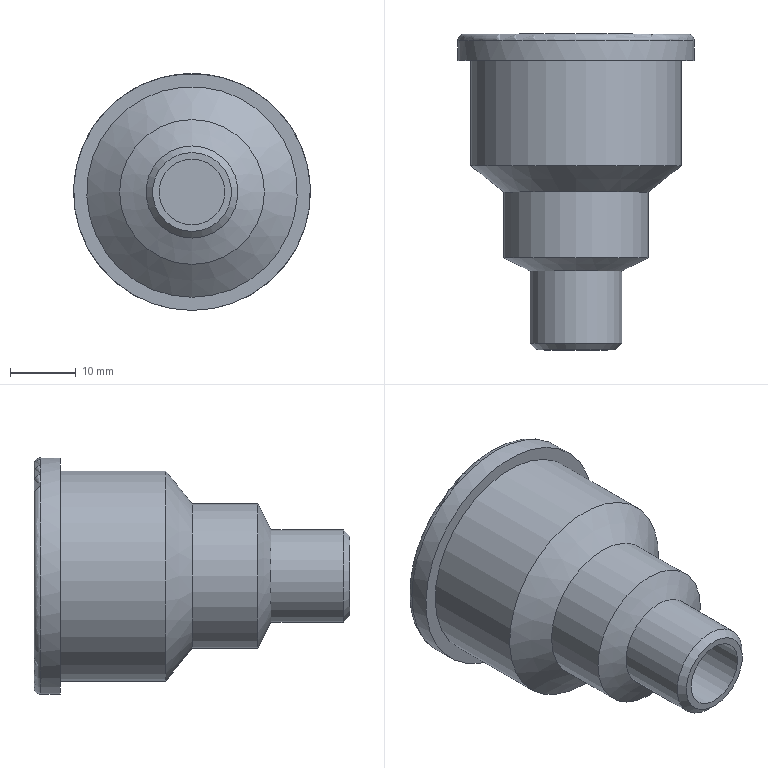Part | NX | features DATUM_CSYS 2, ABSOLUTE_DATUM_PLANE 1, BLEND 1, CHAMFER 1, SHELL 1, SKETCH 1, SWP104 1 | 1 solid | 17 faces | box 36 x 48 x 36 mm | volume 9367 mm3 | cylinder 7 | cone 5 | plane 4 | torus 1 | commonest cylinder face diameters 10 x1 14 x1 18 x1 22 x1 28 x1 32 x1
STEP:
#1=CARTESIAN_POINT('',(0.,-4.,-16.));
#2=VERTEX_POINT('',#1);
#3=CARTESIAN_POINT('',(0.,-4.,0.));
#4=DIRECTION('',(0.,-1.,0.));
#5=DIRECTION('',(0.,0.,-1.));
#6=AXIS2_PLACEMENT_3D('',#3,#4,#5);
#7=CIRCLE('',#6,16.);
#8=EDGE_CURVE('',#2,#2,#7,.T.);
#9=ORIENTED_EDGE('',*,*,#8,.T.);
#10=EDGE_LOOP('',(#9));
#11=FACE_BOUND('',#10,.T.);
#12=CARTESIAN_POINT('',(0.,-20.,-16.));
#13=VERTEX_POINT('',#12);
#14=CARTESIAN_POINT('',(0.,-20.,0.));
#15=DIRECTION('',(0.,-1.,0.));
#16=DIRECTION('',(0.,0.,-1.));
#17=AXIS2_PLACEMENT_3D('',#14,#15,#16);
#18=CIRCLE('',#17,16.);
#19=EDGE_CURVE('',#13,#13,#18,.T.);
#20=ORIENTED_EDGE('',*,*,#19,.F.);
#21=EDGE_LOOP('',(#20));
#22=FACE_BOUND('',#21,.T.);
#23=CARTESIAN_POINT('',(0.,0.,0.));
#24=DIRECTION('',(0.,-1.,0.));
#25=DIRECTION('',(0.,0.,-1.));
#26=AXIS2_PLACEMENT_3D('',#23,#24,#25);
#27=CYLINDRICAL_SURFACE('',#26,16.);
#28=ADVANCED_FACE('',(#11,#22),#27,.T.);
#29=CARTESIAN_POINT('',(0.,-4.,-18.));
#30=VERTEX_POINT('',#29);
#31=CARTESIAN_POINT('',(0.,-4.,0.));
#32=DIRECTION('',(0.,-1.,0.));
#33=DIRECTION('',(0.,0.,-1.));
#34=AXIS2_PLACEMENT_3D('',#31,#32,#33);
#35=CIRCLE('',#34,18.);
#36=EDGE_CURVE('',#30,#30,#35,.T.);
#37=ORIENTED_EDGE('',*,*,#36,.T.);
#38=EDGE_LOOP('',(#37));
#39=FACE_BOUND('',#38,.T.);
#40=ORIENTED_EDGE('',*,*,#8,.F.);
#41=EDGE_LOOP('',(#40));
#42=FACE_BOUND('',#41,.T.);
#43=CARTESIAN_POINT('',(16.,-4.,0.));
#44=DIRECTION('',(0.,-1.,0.));
#45=DIRECTION('',(0.,0.,-1.));
#46=AXIS2_PLACEMENT_3D('',#43,#44,#45);
#47=PLANE('',#46);
#48=ADVANCED_FACE('',(#39,#42),#47,.T.);
#49=CARTESIAN_POINT('',(0.,-1.,18.));
#50=VERTEX_POINT('',#49);
#51=CARTESIAN_POINT('',(0.,-1.,0.));
#52=DIRECTION('',(0.,1.,0.));
#53=DIRECTION('',(0.,0.,1.));
#54=AXIS2_PLACEMENT_3D('',#51,#52,#53);
#55=CIRCLE('',#54,18.);
#56=EDGE_CURVE('',#50,#50,#55,.F.);
#57=ORIENTED_EDGE('',*,*,#56,.T.);
#58=EDGE_LOOP('',(#57));
#59=FACE_BOUND('',#58,.T.);
#60=ORIENTED_EDGE('',*,*,#36,.F.);
#61=EDGE_LOOP('',(#60));
#62=FACE_BOUND('',#61,.T.);
#63=CARTESIAN_POINT('',(0.,0.,0.));
#64=DIRECTION('',(0.,-1.,0.));
#65=DIRECTION('',(0.,0.,-1.));
#66=AXIS2_PLACEMENT_3D('',#63,#64,#65);
#67=CYLINDRICAL_SURFACE('',#66,18.);
#68=ADVANCED_FACE('',(#59,#62),#67,.T.);
#69=CARTESIAN_POINT('',(0.,0.,17.));
#70=VERTEX_POINT('',#69);
#71=CARTESIAN_POINT('',(0.,0.,0.));
#72=DIRECTION('',(0.,1.,0.));
#73=DIRECTION('',(0.,0.,1.));
#74=AXIS2_PLACEMENT_3D('',#71,#72,#73);
#75=CIRCLE('',#74,17.);
#76=EDGE_CURVE('',#70,#70,#75,.T.);
#77=ORIENTED_EDGE('',*,*,#76,.T.);
#78=EDGE_LOOP('',(#77));
#79=FACE_BOUND('',#78,.T.);
#80=CARTESIAN_POINT('',(18.,0.,0.));
#81=DIRECTION('',(0.,1.,0.));
#82=DIRECTION('',(0.,0.,1.));
#83=AXIS2_PLACEMENT_3D('',#80,#81,#82);
#84=PLANE('',#83);
#85=ADVANCED_FACE('',(#79),#84,.T.);
#86=CARTESIAN_POINT('',(0.,-48.,-6.));
#87=VERTEX_POINT('',#86);
#88=CARTESIAN_POINT('',(0.,-48.,0.));
#89=DIRECTION('',(0.,-1.,0.));
#90=DIRECTION('',(0.,0.,-1.));
#91=AXIS2_PLACEMENT_3D('',#88,#89,#90);
#92=CIRCLE('',#91,6.);
#93=EDGE_CURVE('',#87,#87,#92,.T.);
#94=ORIENTED_EDGE('',*,*,#93,.T.);
#95=EDGE_LOOP('',(#94));
#96=FACE_BOUND('',#95,.T.);
#97=CARTESIAN_POINT('',(0.,-48.,-5.));
#98=VERTEX_POINT('',#97);
#99=CARTESIAN_POINT('',(0.,-48.,0.));
#100=DIRECTION('',(0.,-1.,0.));
#101=DIRECTION('',(0.,0.,-1.));
#102=AXIS2_PLACEMENT_3D('',#99,#100,#101);
#103=CIRCLE('',#102,5.);
#104=EDGE_CURVE('',#98,#98,#103,.T.);
#105=ORIENTED_EDGE('',*,*,#104,.F.);
#106=EDGE_LOOP('',(#105));
#107=FACE_BOUND('',#106,.T.);
#108=CARTESIAN_POINT('',(0.,-48.,0.));
#109=DIRECTION('',(0.,-1.,0.));
#110=DIRECTION('',(0.,0.,-1.));
#111=AXIS2_PLACEMENT_3D('',#108,#109,#110);
#112=PLANE('',#111);
#113=ADVANCED_FACE('',(#96,#107),#112,.T.);
#114=CARTESIAN_POINT('',(0.,-47.,-7.));
#115=VERTEX_POINT('',#114);
#116=CARTESIAN_POINT('',(0.,-47.,0.));
#117=DIRECTION('',(0.,-1.,0.));
#118=DIRECTION('',(0.,0.,-1.));
#119=AXIS2_PLACEMENT_3D('',#116,#117,#118);
#120=CIRCLE('',#119,7.);
#121=EDGE_CURVE('',#115,#115,#120,.F.);
#122=ORIENTED_EDGE('',*,*,#121,.T.);
#123=EDGE_LOOP('',(#122));
#124=FACE_BOUND('',#123,.T.);
#125=CARTESIAN_POINT('',(0.,-36.,-7.));
#126=VERTEX_POINT('',#125);
#127=CARTESIAN_POINT('',(0.,-36.,0.));
#128=DIRECTION('',(0.,-1.,0.));
#129=DIRECTION('',(0.,0.,-1.));
#130=AXIS2_PLACEMENT_3D('',#127,#128,#129);
#131=CIRCLE('',#130,7.);
#132=EDGE_CURVE('',#126,#126,#131,.T.);
#133=ORIENTED_EDGE('',*,*,#132,.T.);
#134=EDGE_LOOP('',(#133));
#135=FACE_BOUND('',#134,.T.);
#136=CARTESIAN_POINT('',(0.,0.,0.));
#137=DIRECTION('',(0.,-1.,0.));
#138=DIRECTION('',(0.,0.,-1.));
#139=AXIS2_PLACEMENT_3D('',#136,#137,#138);
#140=CYLINDRICAL_SURFACE('',#139,7.);
#141=ADVANCED_FACE('',(#124,#135),#140,.T.);
#142=CARTESIAN_POINT('',(0.,-34.,-11.));
#143=VERTEX_POINT('',#142);
#144=CARTESIAN_POINT('',(0.,-34.,0.));
#145=DIRECTION('',(0.,-1.,0.));
#146=DIRECTION('',(0.,0.,-1.));
#147=AXIS2_PLACEMENT_3D('',#144,#145,#146);
#148=CIRCLE('',#147,11.);
#149=EDGE_CURVE('',#143,#143,#148,.T.);
#150=ORIENTED_EDGE('',*,*,#149,.T.);
#151=EDGE_LOOP('',(#150));
#152=FACE_BOUND('',#151,.T.);
#153=ORIENTED_EDGE('',*,*,#132,.F.);
#154=EDGE_LOOP('',(#153));
#155=FACE_BOUND('',#154,.T.);
#156=CARTESIAN_POINT('',(0.,-36.,0.));
#157=DIRECTION('',(0.,1.,0.));
#158=DIRECTION('',(0.,0.,1.));
#159=AXIS2_PLACEMENT_3D('',#156,#157,#158);
#160=CONICAL_SURFACE('',#159,7.,1.107);
#161=ADVANCED_FACE('',(#152,#155),#160,.T.);
#162=CARTESIAN_POINT('',(0.,-24.,-11.));
#163=VERTEX_POINT('',#162);
#164=CARTESIAN_POINT('',(0.,-24.,0.));
#165=DIRECTION('',(0.,-1.,0.));
#166=DIRECTION('',(0.,0.,-1.));
#167=AXIS2_PLACEMENT_3D('',#164,#165,#166);
#168=CIRCLE('',#167,11.);
#169=EDGE_CURVE('',#163,#163,#168,.T.);
#170=ORIENTED_EDGE('',*,*,#169,.T.);
#171=EDGE_LOOP('',(#170));
#172=FACE_BOUND('',#171,.T.);
#173=ORIENTED_EDGE('',*,*,#149,.F.);
#174=EDGE_LOOP('',(#173));
#175=FACE_BOUND('',#174,.T.);
#176=CARTESIAN_POINT('',(0.,0.,0.));
#177=DIRECTION('',(0.,-1.,0.));
#178=DIRECTION('',(0.,0.,-1.));
#179=AXIS2_PLACEMENT_3D('',#176,#177,#178);
#180=CYLINDRICAL_SURFACE('',#179,11.);
#181=ADVANCED_FACE('',(#172,#175),#180,.T.);
#182=ORIENTED_EDGE('',*,*,#19,.T.);
#183=EDGE_LOOP('',(#182));
#184=FACE_BOUND('',#183,.T.);
#185=ORIENTED_EDGE('',*,*,#169,.F.);
#186=EDGE_LOOP('',(#185));
#187=FACE_BOUND('',#186,.T.);
#188=CARTESIAN_POINT('',(0.,-24.,0.));
#189=DIRECTION('',(0.,1.,0.));
#190=DIRECTION('',(0.,0.,1.));
#191=AXIS2_PLACEMENT_3D('',#188,#189,#190);
#192=CONICAL_SURFACE('',#191,11.,0.8961);
#193=ADVANCED_FACE('',(#184,#187),#192,.T.);
#194=CARTESIAN_POINT('',(0.,-2.,-14.));
#195=VERTEX_POINT('',#194);
#196=CARTESIAN_POINT('',(0.,-2.,0.));
#197=DIRECTION('',(0.,-1.,0.));
#198=DIRECTION('',(0.,0.,-1.));
#199=AXIS2_PLACEMENT_3D('',#196,#197,#198);
#200=CIRCLE('',#199,14.);
#201=EDGE_CURVE('',#195,#195,#200,.T.);
#202=ORIENTED_EDGE('',*,*,#201,.F.);
#203=EDGE_LOOP('',(#202));
#204=FACE_BOUND('',#203,.T.);
#205=CARTESIAN_POINT('',(0.,-19.039,14.));
#206=VERTEX_POINT('',#205);
#207=CARTESIAN_POINT('',(0.,-19.039,0.));
#208=DIRECTION('',(0.,1.,0.));
#209=DIRECTION('',(0.,0.,1.));
#210=AXIS2_PLACEMENT_3D('',#207,#208,#209);
#211=CIRCLE('',#210,14.);
#212=EDGE_CURVE('',#206,#206,#211,.F.);
#213=ORIENTED_EDGE('',*,*,#212,.T.);
#214=EDGE_LOOP('',(#213));
#215=FACE_BOUND('',#214,.T.);
#216=CARTESIAN_POINT('',(0.,0.,0.));
#217=DIRECTION('',(0.,-1.,0.));
#218=DIRECTION('',(0.,0.,-1.));
#219=AXIS2_PLACEMENT_3D('',#216,#217,#218);
#220=CYLINDRICAL_SURFACE('',#219,14.);
#221=ADVANCED_FACE('',(#204,#215),#220,.F.);
#222=ORIENTED_EDGE('',*,*,#201,.T.);
#223=EDGE_LOOP('',(#222));
#224=FACE_BOUND('',#223,.T.);
#225=CARTESIAN_POINT('',(18.,-2.,0.));
#226=DIRECTION('',(0.,1.,0.));
#227=DIRECTION('',(0.,0.,1.));
#228=AXIS2_PLACEMENT_3D('',#225,#226,#227);
#229=PLANE('',#228);
#230=ADVANCED_FACE('',(#224),#229,.F.);
#231=CARTESIAN_POINT('',(0.,-34.764,5.));
#232=VERTEX_POINT('',#231);
#233=CARTESIAN_POINT('',(0.,-34.764,0.));
#234=DIRECTION('',(0.,1.,0.));
#235=DIRECTION('',(0.,0.,1.));
#236=AXIS2_PLACEMENT_3D('',#233,#234,#235);
#237=CIRCLE('',#236,5.);
#238=EDGE_CURVE('',#232,#232,#237,.F.);
#239=ORIENTED_EDGE('',*,*,#238,.F.);
#240=EDGE_LOOP('',(#239));
#241=FACE_BOUND('',#240,.T.);
#242=ORIENTED_EDGE('',*,*,#104,.T.);
#243=EDGE_LOOP('',(#242));
#244=FACE_BOUND('',#243,.T.);
#245=CARTESIAN_POINT('',(0.,0.,0.));
#246=DIRECTION('',(0.,-1.,0.));
#247=DIRECTION('',(0.,0.,-1.));
#248=AXIS2_PLACEMENT_3D('',#245,#246,#247);
#249=CYLINDRICAL_SURFACE('',#248,5.);
#250=ADVANCED_FACE('',(#241,#244),#249,.F.);
#251=CARTESIAN_POINT('',(0.,-32.764,9.));
#252=VERTEX_POINT('',#251);
#253=CARTESIAN_POINT('',(0.,-32.764,0.));
#254=DIRECTION('',(0.,1.,0.));
#255=DIRECTION('',(0.,0.,1.));
#256=AXIS2_PLACEMENT_3D('',#253,#254,#255);
#257=CIRCLE('',#256,9.);
#258=EDGE_CURVE('',#252,#252,#257,.F.);
#259=ORIENTED_EDGE('',*,*,#258,.F.);
#260=EDGE_LOOP('',(#259));
#261=FACE_BOUND('',#260,.T.);
#262=ORIENTED_EDGE('',*,*,#238,.T.);
#263=EDGE_LOOP('',(#262));
#264=FACE_BOUND('',#263,.T.);
#265=CARTESIAN_POINT('',(0.,-34.211,0.));
#266=DIRECTION('',(0.,1.,0.));
#267=DIRECTION('',(0.,0.,1.));
#268=AXIS2_PLACEMENT_3D('',#265,#266,#267);
#269=CONICAL_SURFACE('',#268,6.106,1.107);
#270=ADVANCED_FACE('',(#261,#264),#269,.F.);
#271=CARTESIAN_POINT('',(0.,-23.039,9.));
#272=VERTEX_POINT('',#271);
#273=CARTESIAN_POINT('',(0.,-23.039,0.));
#274=DIRECTION('',(0.,1.,0.));
#275=DIRECTION('',(0.,0.,1.));
#276=AXIS2_PLACEMENT_3D('',#273,#274,#275);
#277=CIRCLE('',#276,9.);
#278=EDGE_CURVE('',#272,#272,#277,.F.);
#279=ORIENTED_EDGE('',*,*,#278,.F.);
#280=EDGE_LOOP('',(#279));
#281=FACE_BOUND('',#280,.T.);
#282=ORIENTED_EDGE('',*,*,#258,.T.);
#283=EDGE_LOOP('',(#282));
#284=FACE_BOUND('',#283,.T.);
#285=CARTESIAN_POINT('',(0.,0.,0.));
#286=DIRECTION('',(0.,-1.,0.));
#287=DIRECTION('',(0.,0.,-1.));
#288=AXIS2_PLACEMENT_3D('',#285,#286,#287);
#289=CYLINDRICAL_SURFACE('',#288,9.);
#290=ADVANCED_FACE('',(#281,#284),#289,.F.);
#291=ORIENTED_EDGE('',*,*,#212,.F.);
#292=EDGE_LOOP('',(#291));
#293=FACE_BOUND('',#292,.T.);
#294=ORIENTED_EDGE('',*,*,#278,.T.);
#295=EDGE_LOOP('',(#294));
#296=FACE_BOUND('',#295,.T.);
#297=CARTESIAN_POINT('',(0.,-22.438,0.));
#298=DIRECTION('',(0.,1.,0.));
#299=DIRECTION('',(0.,0.,1.));
#300=AXIS2_PLACEMENT_3D('',#297,#298,#299);
#301=CONICAL_SURFACE('',#300,9.751,0.8961);
#302=ADVANCED_FACE('',(#293,#296),#301,.F.);
#303=ORIENTED_EDGE('',*,*,#76,.F.);
#304=EDGE_LOOP('',(#303));
#305=FACE_BOUND('',#304,.T.);
#306=ORIENTED_EDGE('',*,*,#56,.F.);
#307=EDGE_LOOP('',(#306));
#308=FACE_BOUND('',#307,.T.);
#309=CARTESIAN_POINT('',(0.,-1.,0.));
#310=DIRECTION('',(0.,1.,0.));
#311=DIRECTION('',(0.,0.,1.));
#312=AXIS2_PLACEMENT_3D('',#309,#310,#311);
#313=TOROIDAL_SURFACE('',#312,17.,1.);
#314=ADVANCED_FACE('',(#305,#308),#313,.T.);
#315=ORIENTED_EDGE('',*,*,#121,.F.);
#316=EDGE_LOOP('',(#315));
#317=FACE_BOUND('',#316,.T.);
#318=ORIENTED_EDGE('',*,*,#93,.F.);
#319=EDGE_LOOP('',(#318));
#320=FACE_BOUND('',#319,.T.);
#321=CARTESIAN_POINT('',(0.,-48.,0.));
#322=DIRECTION('',(0.,1.,0.));
#323=DIRECTION('',(0.,0.,1.));
#324=AXIS2_PLACEMENT_3D('',#321,#322,#323);
#325=CONICAL_SURFACE('',#324,6.,0.7854);
#326=ADVANCED_FACE('',(#317,#320),#325,.T.);
#327=CLOSED_SHELL('',(#28,#48,#68,#85,#113,#141,#161,#181,#193,#221,#230,#250,#270,#290,#302,#314,#326));
#328=MANIFOLD_SOLID_BREP('',#327);
#329=(LENGTH_UNIT()NAMED_UNIT(*)SI_UNIT(.MILLI.,.METRE.));
#330=UNCERTAINTY_MEASURE_WITH_UNIT(LENGTH_MEASURE(0.00001),#329,'','');
#331=(NAMED_UNIT(*)PLANE_ANGLE_UNIT()SI_UNIT($,.RADIAN.));
#332=(NAMED_UNIT(*)SI_UNIT($,.STERADIAN.)SOLID_ANGLE_UNIT());
#333=(GEOMETRIC_REPRESENTATION_CONTEXT(3)GLOBAL_UNCERTAINTY_ASSIGNED_CONTEXT((#330))GLOBAL_UNIT_ASSIGNED_CONTEXT((#329,#331,#332))REPRESENTATION_CONTEXT('',''));
#334=ADVANCED_BREP_SHAPE_REPRESENTATION('',(#328),#333);